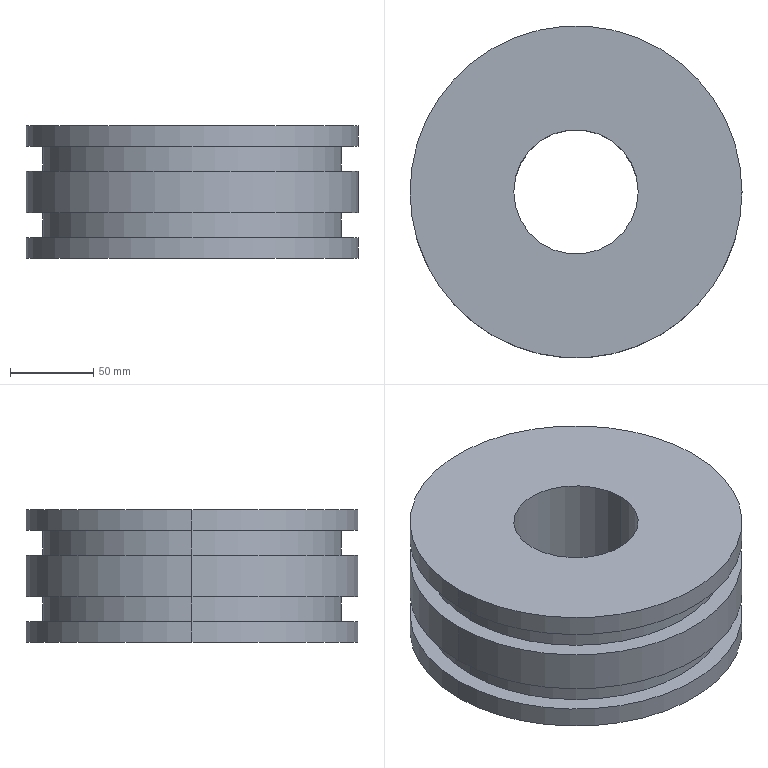Part | SolidWorks | features Extrusion 1, ICE 1, MirrorPattern 1 | 1 solid | 18 faces | box 200 x 200 x 80 mm | volume 1980774 mm3 | cylinder 12 | plane 6 | commonest cylinder face diameters 200 x6 180 x4 75 x2
STEP:
#1=CARTESIAN_POINT('',(90.,0.,-12.5));
#2=VERTEX_POINT('',#1);
#3=CARTESIAN_POINT('',(-90.,0.,-12.5));
#4=VERTEX_POINT('',#3);
#5=CARTESIAN_POINT('',(0.,0.,-12.5));
#6=DIRECTION('',(0.,0.,1.));
#7=DIRECTION('',(1.,0.,0.));
#8=AXIS2_PLACEMENT_3D('',#5,#6,#7);
#9=CIRCLE('',#8,90.);
#10=EDGE_CURVE('',#2,#4,#9,.T.);
#11=ORIENTED_EDGE('',*,*,#10,.F.);
#12=CARTESIAN_POINT('',(90.,0.,-27.5));
#13=VERTEX_POINT('',#12);
#14=CARTESIAN_POINT('',(90.,0.,-12.5));
#15=DIRECTION('',(0.,0.,-1.));
#16=VECTOR('',#15,1000.);
#17=LINE('',#14,#16);
#18=EDGE_CURVE('',#2,#13,#17,.T.);
#19=ORIENTED_EDGE('',*,*,#18,.T.);
#20=CARTESIAN_POINT('',(-90.,0.,-27.5));
#21=VERTEX_POINT('',#20);
#22=CARTESIAN_POINT('',(0.,0.,-27.5));
#23=DIRECTION('',(0.,0.,1.));
#24=DIRECTION('',(1.,0.,0.));
#25=AXIS2_PLACEMENT_3D('',#22,#23,#24);
#26=CIRCLE('',#25,90.);
#27=EDGE_CURVE('',#13,#21,#26,.T.);
#28=ORIENTED_EDGE('',*,*,#27,.T.);
#29=CARTESIAN_POINT('',(-90.,0.,-12.5));
#30=DIRECTION('',(0.,0.,-1.));
#31=VECTOR('',#30,1000.);
#32=LINE('',#29,#31);
#33=EDGE_CURVE('',#4,#21,#32,.T.);
#34=ORIENTED_EDGE('',*,*,#33,.F.);
#35=EDGE_LOOP('',(#11,#19,#28,#34));
#36=FACE_OUTER_BOUND('',#35,.T.);
#37=CARTESIAN_POINT('',(0.,0.,-12.5));
#38=DIRECTION('',(0.,0.,-1.));
#39=DIRECTION('',(-1.,0.,0.));
#40=AXIS2_PLACEMENT_3D('',#37,#38,#39);
#41=CYLINDRICAL_SURFACE('',#40,90.);
#42=ADVANCED_FACE('',(#36),#41,.T.);
#43=CARTESIAN_POINT('',(90.,0.,12.5));
#44=VERTEX_POINT('',#43);
#45=CARTESIAN_POINT('',(-90.,0.,12.5));
#46=VERTEX_POINT('',#45);
#47=CARTESIAN_POINT('',(0.,0.,12.5));
#48=DIRECTION('',(0.,0.,1.));
#49=DIRECTION('',(1.,0.,0.));
#50=AXIS2_PLACEMENT_3D('',#47,#48,#49);
#51=CIRCLE('',#50,90.);
#52=EDGE_CURVE('',#44,#46,#51,.T.);
#53=ORIENTED_EDGE('',*,*,#52,.T.);
#54=CARTESIAN_POINT('',(-90.,0.,27.5));
#55=VERTEX_POINT('',#54);
#56=CARTESIAN_POINT('',(-90.,0.,12.5));
#57=DIRECTION('',(0.,0.,1.));
#58=VECTOR('',#57,1000.);
#59=LINE('',#56,#58);
#60=EDGE_CURVE('',#46,#55,#59,.T.);
#61=ORIENTED_EDGE('',*,*,#60,.T.);
#62=CARTESIAN_POINT('',(90.,0.,27.5));
#63=VERTEX_POINT('',#62);
#64=CARTESIAN_POINT('',(0.,0.,27.5));
#65=DIRECTION('',(0.,0.,1.));
#66=DIRECTION('',(1.,0.,0.));
#67=AXIS2_PLACEMENT_3D('',#64,#65,#66);
#68=CIRCLE('',#67,90.);
#69=EDGE_CURVE('',#63,#55,#68,.T.);
#70=ORIENTED_EDGE('',*,*,#69,.F.);
#71=CARTESIAN_POINT('',(90.,0.,12.5));
#72=DIRECTION('',(0.,0.,1.));
#73=VECTOR('',#72,1000.);
#74=LINE('',#71,#73);
#75=EDGE_CURVE('',#44,#63,#74,.T.);
#76=ORIENTED_EDGE('',*,*,#75,.F.);
#77=EDGE_LOOP('',(#53,#61,#70,#76));
#78=FACE_OUTER_BOUND('',#77,.T.);
#79=CARTESIAN_POINT('',(0.,0.,12.5));
#80=DIRECTION('',(0.,0.,1.));
#81=DIRECTION('',(1.,0.,0.));
#82=AXIS2_PLACEMENT_3D('',#79,#80,#81);
#83=CYLINDRICAL_SURFACE('',#82,90.);
#84=ADVANCED_FACE('',(#78),#83,.T.);
#85=CARTESIAN_POINT('',(-37.5,0.,40.));
#86=VERTEX_POINT('',#85);
#87=CARTESIAN_POINT('',(37.5,0.,40.));
#88=VERTEX_POINT('',#87);
#89=CARTESIAN_POINT('',(0.,0.,40.));
#90=DIRECTION('',(0.,0.,1.));
#91=DIRECTION('',(1.,0.,0.));
#92=AXIS2_PLACEMENT_3D('',#89,#90,#91);
#93=CIRCLE('',#92,37.5);
#94=EDGE_CURVE('',#86,#88,#93,.T.);
#95=ORIENTED_EDGE('',*,*,#94,.T.);
#96=CARTESIAN_POINT('',(37.5,0.,-40.));
#97=VERTEX_POINT('',#96);
#98=CARTESIAN_POINT('',(37.5,0.,40.));
#99=DIRECTION('',(0.,0.,-1.));
#100=VECTOR('',#99,1000.);
#101=LINE('',#98,#100);
#102=EDGE_CURVE('',#88,#97,#101,.T.);
#103=ORIENTED_EDGE('',*,*,#102,.T.);
#104=CARTESIAN_POINT('',(-37.5,0.,-40.));
#105=VERTEX_POINT('',#104);
#106=CARTESIAN_POINT('',(0.,0.,-40.));
#107=DIRECTION('',(0.,0.,1.));
#108=DIRECTION('',(1.,0.,0.));
#109=AXIS2_PLACEMENT_3D('',#106,#107,#108);
#110=CIRCLE('',#109,37.5);
#111=EDGE_CURVE('',#105,#97,#110,.T.);
#112=ORIENTED_EDGE('',*,*,#111,.F.);
#113=CARTESIAN_POINT('',(-37.5,0.,40.));
#114=DIRECTION('',(0.,0.,-1.));
#115=VECTOR('',#114,1000.);
#116=LINE('',#113,#115);
#117=EDGE_CURVE('',#86,#105,#116,.T.);
#118=ORIENTED_EDGE('',*,*,#117,.F.);
#119=EDGE_LOOP('',(#95,#103,#112,#118));
#120=FACE_OUTER_BOUND('',#119,.T.);
#121=CARTESIAN_POINT('',(0.,0.,40.));
#122=DIRECTION('',(0.,0.,-1.));
#123=DIRECTION('',(-1.,0.,0.));
#124=AXIS2_PLACEMENT_3D('',#121,#122,#123);
#125=CYLINDRICAL_SURFACE('',#124,37.5);
#126=ADVANCED_FACE('',(#120),#125,.F.);
#127=CARTESIAN_POINT('',(100.,0.,40.));
#128=VERTEX_POINT('',#127);
#129=CARTESIAN_POINT('',(-100.,0.,40.));
#130=VERTEX_POINT('',#129);
#131=CARTESIAN_POINT('',(0.,0.,40.));
#132=DIRECTION('',(0.,0.,1.));
#133=DIRECTION('',(1.,0.,0.));
#134=AXIS2_PLACEMENT_3D('',#131,#132,#133);
#135=CIRCLE('',#134,100.);
#136=EDGE_CURVE('',#128,#130,#135,.T.);
#137=ORIENTED_EDGE('',*,*,#136,.F.);
#138=CARTESIAN_POINT('',(100.,0.,27.5));
#139=VERTEX_POINT('',#138);
#140=CARTESIAN_POINT('',(100.,0.,40.));
#141=DIRECTION('',(0.,0.,-1.));
#142=VECTOR('',#141,1000.);
#143=LINE('',#140,#142);
#144=EDGE_CURVE('',#128,#139,#143,.T.);
#145=ORIENTED_EDGE('',*,*,#144,.T.);
#146=CARTESIAN_POINT('',(-100.,0.,27.5));
#147=VERTEX_POINT('',#146);
#148=CARTESIAN_POINT('',(0.,0.,27.5));
#149=DIRECTION('',(0.,0.,1.));
#150=DIRECTION('',(1.,0.,0.));
#151=AXIS2_PLACEMENT_3D('',#148,#149,#150);
#152=CIRCLE('',#151,100.);
#153=EDGE_CURVE('',#139,#147,#152,.T.);
#154=ORIENTED_EDGE('',*,*,#153,.T.);
#155=CARTESIAN_POINT('',(-100.,0.,40.));
#156=DIRECTION('',(0.,0.,-1.));
#157=VECTOR('',#156,1000.);
#158=LINE('',#155,#157);
#159=EDGE_CURVE('',#130,#147,#158,.T.);
#160=ORIENTED_EDGE('',*,*,#159,.F.);
#161=EDGE_LOOP('',(#137,#145,#154,#160));
#162=FACE_OUTER_BOUND('',#161,.T.);
#163=CARTESIAN_POINT('',(0.,0.,40.));
#164=DIRECTION('',(0.,0.,-1.));
#165=DIRECTION('',(-1.,0.,0.));
#166=AXIS2_PLACEMENT_3D('',#163,#164,#165);
#167=CYLINDRICAL_SURFACE('',#166,100.);
#168=ADVANCED_FACE('',(#162),#167,.T.);
#169=CARTESIAN_POINT('',(100.,0.,-27.5));
#170=VERTEX_POINT('',#169);
#171=CARTESIAN_POINT('',(-100.,0.,-27.5));
#172=VERTEX_POINT('',#171);
#173=CARTESIAN_POINT('',(0.,0.,-27.5));
#174=DIRECTION('',(0.,0.,1.));
#175=DIRECTION('',(1.,0.,0.));
#176=AXIS2_PLACEMENT_3D('',#173,#174,#175);
#177=CIRCLE('',#176,100.);
#178=EDGE_CURVE('',#170,#172,#177,.T.);
#179=ORIENTED_EDGE('',*,*,#178,.F.);
#180=CARTESIAN_POINT('',(100.,0.,-40.));
#181=VERTEX_POINT('',#180);
#182=CARTESIAN_POINT('',(100.,0.,40.));
#183=DIRECTION('',(0.,0.,-1.));
#184=VECTOR('',#183,1000.);
#185=LINE('',#182,#184);
#186=EDGE_CURVE('',#170,#181,#185,.T.);
#187=ORIENTED_EDGE('',*,*,#186,.T.);
#188=CARTESIAN_POINT('',(-100.,0.,-40.));
#189=VERTEX_POINT('',#188);
#190=CARTESIAN_POINT('',(0.,0.,-40.));
#191=DIRECTION('',(0.,0.,1.));
#192=DIRECTION('',(1.,0.,0.));
#193=AXIS2_PLACEMENT_3D('',#190,#191,#192);
#194=CIRCLE('',#193,100.);
#195=EDGE_CURVE('',#181,#189,#194,.T.);
#196=ORIENTED_EDGE('',*,*,#195,.T.);
#197=CARTESIAN_POINT('',(-100.,0.,40.));
#198=DIRECTION('',(0.,0.,-1.));
#199=VECTOR('',#198,1000.);
#200=LINE('',#197,#199);
#201=EDGE_CURVE('',#172,#189,#200,.T.);
#202=ORIENTED_EDGE('',*,*,#201,.F.);
#203=EDGE_LOOP('',(#179,#187,#196,#202));
#204=FACE_OUTER_BOUND('',#203,.T.);
#205=CARTESIAN_POINT('',(0.,0.,40.));
#206=DIRECTION('',(0.,0.,-1.));
#207=DIRECTION('',(-1.,0.,0.));
#208=AXIS2_PLACEMENT_3D('',#205,#206,#207);
#209=CYLINDRICAL_SURFACE('',#208,100.);
#210=ADVANCED_FACE('',(#204),#209,.T.);
#211=CARTESIAN_POINT('',(100.,0.,12.5));
#212=VERTEX_POINT('',#211);
#213=CARTESIAN_POINT('',(-100.,0.,12.5));
#214=VERTEX_POINT('',#213);
#215=CARTESIAN_POINT('',(0.,0.,12.5));
#216=DIRECTION('',(0.,0.,1.));
#217=DIRECTION('',(1.,0.,0.));
#218=AXIS2_PLACEMENT_3D('',#215,#216,#217);
#219=CIRCLE('',#218,100.);
#220=EDGE_CURVE('',#212,#214,#219,.T.);
#221=ORIENTED_EDGE('',*,*,#220,.F.);
#222=CARTESIAN_POINT('',(100.,0.,-12.5));
#223=VERTEX_POINT('',#222);
#224=CARTESIAN_POINT('',(100.,0.,40.));
#225=DIRECTION('',(0.,0.,-1.));
#226=VECTOR('',#225,1000.);
#227=LINE('',#224,#226);
#228=EDGE_CURVE('',#212,#223,#227,.T.);
#229=ORIENTED_EDGE('',*,*,#228,.T.);
#230=CARTESIAN_POINT('',(-100.,0.,-12.5));
#231=VERTEX_POINT('',#230);
#232=CARTESIAN_POINT('',(0.,0.,-12.5));
#233=DIRECTION('',(0.,0.,1.));
#234=DIRECTION('',(1.,0.,0.));
#235=AXIS2_PLACEMENT_3D('',#232,#233,#234);
#236=CIRCLE('',#235,100.);
#237=EDGE_CURVE('',#223,#231,#236,.T.);
#238=ORIENTED_EDGE('',*,*,#237,.T.);
#239=CARTESIAN_POINT('',(-100.,0.,40.));
#240=DIRECTION('',(0.,0.,-1.));
#241=VECTOR('',#240,1000.);
#242=LINE('',#239,#241);
#243=EDGE_CURVE('',#214,#231,#242,.T.);
#244=ORIENTED_EDGE('',*,*,#243,.F.);
#245=EDGE_LOOP('',(#221,#229,#238,#244));
#246=FACE_OUTER_BOUND('',#245,.T.);
#247=CARTESIAN_POINT('',(0.,0.,40.));
#248=DIRECTION('',(0.,0.,-1.));
#249=DIRECTION('',(-1.,0.,0.));
#250=AXIS2_PLACEMENT_3D('',#247,#248,#249);
#251=CYLINDRICAL_SURFACE('',#250,100.);
#252=ADVANCED_FACE('',(#246),#251,.T.);
#253=ORIENTED_EDGE('',*,*,#228,.F.);
#254=CARTESIAN_POINT('',(0.,0.,12.5));
#255=DIRECTION('',(0.,0.,1.));
#256=DIRECTION('',(1.,0.,0.));
#257=AXIS2_PLACEMENT_3D('',#254,#255,#256);
#258=CIRCLE('',#257,100.);
#259=EDGE_CURVE('',#214,#212,#258,.T.);
#260=ORIENTED_EDGE('',*,*,#259,.F.);
#261=ORIENTED_EDGE('',*,*,#243,.T.);
#262=CARTESIAN_POINT('',(0.,0.,-12.5));
#263=DIRECTION('',(0.,0.,1.));
#264=DIRECTION('',(1.,0.,0.));
#265=AXIS2_PLACEMENT_3D('',#262,#263,#264);
#266=CIRCLE('',#265,100.);
#267=EDGE_CURVE('',#231,#223,#266,.T.);
#268=ORIENTED_EDGE('',*,*,#267,.T.);
#269=EDGE_LOOP('',(#253,#260,#261,#268));
#270=FACE_OUTER_BOUND('',#269,.T.);
#271=CARTESIAN_POINT('',(0.,0.,40.));
#272=DIRECTION('',(0.,0.,-1.));
#273=DIRECTION('',(-1.,0.,0.));
#274=AXIS2_PLACEMENT_3D('',#271,#272,#273);
#275=CYLINDRICAL_SURFACE('',#274,100.);
#276=ADVANCED_FACE('',(#270),#275,.T.);
#277=ORIENTED_EDGE('',*,*,#186,.F.);
#278=CARTESIAN_POINT('',(0.,0.,-27.5));
#279=DIRECTION('',(0.,0.,1.));
#280=DIRECTION('',(1.,0.,0.));
#281=AXIS2_PLACEMENT_3D('',#278,#279,#280);
#282=CIRCLE('',#281,100.);
#283=EDGE_CURVE('',#172,#170,#282,.T.);
#284=ORIENTED_EDGE('',*,*,#283,.F.);
#285=ORIENTED_EDGE('',*,*,#201,.T.);
#286=CARTESIAN_POINT('',(0.,0.,-40.));
#287=DIRECTION('',(0.,0.,1.));
#288=DIRECTION('',(1.,0.,0.));
#289=AXIS2_PLACEMENT_3D('',#286,#287,#288);
#290=CIRCLE('',#289,100.);
#291=EDGE_CURVE('',#189,#181,#290,.T.);
#292=ORIENTED_EDGE('',*,*,#291,.T.);
#293=EDGE_LOOP('',(#277,#284,#285,#292));
#294=FACE_OUTER_BOUND('',#293,.T.);
#295=CARTESIAN_POINT('',(0.,0.,40.));
#296=DIRECTION('',(0.,0.,-1.));
#297=DIRECTION('',(-1.,0.,0.));
#298=AXIS2_PLACEMENT_3D('',#295,#296,#297);
#299=CYLINDRICAL_SURFACE('',#298,100.);
#300=ADVANCED_FACE('',(#294),#299,.T.);
#301=CARTESIAN_POINT('',(0.,0.,40.));
#302=DIRECTION('',(0.,0.,1.));
#303=DIRECTION('',(1.,0.,0.));
#304=AXIS2_PLACEMENT_3D('',#301,#302,#303);
#305=CIRCLE('',#304,100.);
#306=EDGE_CURVE('',#130,#128,#305,.T.);
#307=ORIENTED_EDGE('',*,*,#306,.T.);
#308=ORIENTED_EDGE('',*,*,#136,.T.);
#309=EDGE_LOOP('',(#307,#308));
#310=FACE_OUTER_BOUND('',#309,.T.);
#311=ORIENTED_EDGE('',*,*,#94,.F.);
#312=CARTESIAN_POINT('',(0.,0.,40.));
#313=DIRECTION('',(0.,0.,1.));
#314=DIRECTION('',(1.,0.,0.));
#315=AXIS2_PLACEMENT_3D('',#312,#313,#314);
#316=CIRCLE('',#315,37.5);
#317=EDGE_CURVE('',#88,#86,#316,.T.);
#318=ORIENTED_EDGE('',*,*,#317,.F.);
#319=EDGE_LOOP('',(#311,#318));
#320=FACE_BOUND('',#319,.T.);
#321=CARTESIAN_POINT('',(0.,0.,40.));
#322=DIRECTION('',(0.,0.,1.));
#323=DIRECTION('',(1.,0.,0.));
#324=AXIS2_PLACEMENT_3D('',#321,#322,#323);
#325=PLANE('',#324);
#326=ADVANCED_FACE('',(#310,#320),#325,.T.);
#327=ORIENTED_EDGE('',*,*,#291,.F.);
#328=ORIENTED_EDGE('',*,*,#195,.F.);
#329=EDGE_LOOP('',(#327,#328));
#330=FACE_OUTER_BOUND('',#329,.T.);
#331=ORIENTED_EDGE('',*,*,#111,.T.);
#332=CARTESIAN_POINT('',(0.,0.,-40.));
#333=DIRECTION('',(0.,0.,1.));
#334=DIRECTION('',(1.,0.,0.));
#335=AXIS2_PLACEMENT_3D('',#332,#333,#334);
#336=CIRCLE('',#335,37.5);
#337=EDGE_CURVE('',#97,#105,#336,.T.);
#338=ORIENTED_EDGE('',*,*,#337,.T.);
#339=EDGE_LOOP('',(#331,#338));
#340=FACE_BOUND('',#339,.T.);
#341=CARTESIAN_POINT('',(0.,0.,-40.));
#342=DIRECTION('',(0.,0.,1.));
#343=DIRECTION('',(1.,0.,0.));
#344=AXIS2_PLACEMENT_3D('',#341,#342,#343);
#345=PLANE('',#344);
#346=ADVANCED_FACE('',(#330,#340),#345,.F.);
#347=ORIENTED_EDGE('',*,*,#144,.F.);
#348=ORIENTED_EDGE('',*,*,#306,.F.);
#349=ORIENTED_EDGE('',*,*,#159,.T.);
#350=CARTESIAN_POINT('',(0.,0.,27.5));
#351=DIRECTION('',(0.,0.,1.));
#352=DIRECTION('',(1.,0.,0.));
#353=AXIS2_PLACEMENT_3D('',#350,#351,#352);
#354=CIRCLE('',#353,100.);
#355=EDGE_CURVE('',#147,#139,#354,.T.);
#356=ORIENTED_EDGE('',*,*,#355,.T.);
#357=EDGE_LOOP('',(#347,#348,#349,#356));
#358=FACE_OUTER_BOUND('',#357,.T.);
#359=CARTESIAN_POINT('',(0.,0.,40.));
#360=DIRECTION('',(0.,0.,-1.));
#361=DIRECTION('',(-1.,0.,0.));
#362=AXIS2_PLACEMENT_3D('',#359,#360,#361);
#363=CYLINDRICAL_SURFACE('',#362,100.);
#364=ADVANCED_FACE('',(#358),#363,.T.);
#365=ORIENTED_EDGE('',*,*,#102,.F.);
#366=ORIENTED_EDGE('',*,*,#317,.T.);
#367=ORIENTED_EDGE('',*,*,#117,.T.);
#368=ORIENTED_EDGE('',*,*,#337,.F.);
#369=EDGE_LOOP('',(#365,#366,#367,#368));
#370=FACE_OUTER_BOUND('',#369,.T.);
#371=CARTESIAN_POINT('',(0.,0.,40.));
#372=DIRECTION('',(0.,0.,-1.));
#373=DIRECTION('',(-1.,0.,0.));
#374=AXIS2_PLACEMENT_3D('',#371,#372,#373);
#375=CYLINDRICAL_SURFACE('',#374,37.5);
#376=ADVANCED_FACE('',(#370),#375,.F.);
#377=ORIENTED_EDGE('',*,*,#52,.F.);
#378=CARTESIAN_POINT('',(0.,0.,12.5));
#379=DIRECTION('',(0.,0.,1.));
#380=DIRECTION('',(1.,0.,0.));
#381=AXIS2_PLACEMENT_3D('',#378,#379,#380);
#382=CIRCLE('',#381,90.);
#383=EDGE_CURVE('',#46,#44,#382,.T.);
#384=ORIENTED_EDGE('',*,*,#383,.F.);
#385=EDGE_LOOP('',(#377,#384));
#386=FACE_BOUND('',#385,.T.);
#387=ORIENTED_EDGE('',*,*,#259,.T.);
#388=ORIENTED_EDGE('',*,*,#220,.T.);
#389=EDGE_LOOP('',(#387,#388));
#390=FACE_OUTER_BOUND('',#389,.T.);
#391=CARTESIAN_POINT('',(0.,0.,12.5));
#392=DIRECTION('',(0.,0.,1.));
#393=DIRECTION('',(1.,0.,0.));
#394=AXIS2_PLACEMENT_3D('',#391,#392,#393);
#395=PLANE('',#394);
#396=ADVANCED_FACE('',(#386,#390),#395,.T.);
#397=ORIENTED_EDGE('',*,*,#69,.T.);
#398=CARTESIAN_POINT('',(0.,0.,27.5));
#399=DIRECTION('',(0.,0.,1.));
#400=DIRECTION('',(1.,0.,0.));
#401=AXIS2_PLACEMENT_3D('',#398,#399,#400);
#402=CIRCLE('',#401,90.);
#403=EDGE_CURVE('',#55,#63,#402,.T.);
#404=ORIENTED_EDGE('',*,*,#403,.T.);
#405=EDGE_LOOP('',(#397,#404));
#406=FACE_BOUND('',#405,.T.);
#407=ORIENTED_EDGE('',*,*,#355,.F.);
#408=ORIENTED_EDGE('',*,*,#153,.F.);
#409=EDGE_LOOP('',(#407,#408));
#410=FACE_OUTER_BOUND('',#409,.T.);
#411=CARTESIAN_POINT('',(0.,0.,27.5));
#412=DIRECTION('',(0.,0.,1.));
#413=DIRECTION('',(1.,0.,0.));
#414=AXIS2_PLACEMENT_3D('',#411,#412,#413);
#415=PLANE('',#414);
#416=ADVANCED_FACE('',(#406,#410),#415,.F.);
#417=ORIENTED_EDGE('',*,*,#60,.F.);
#418=ORIENTED_EDGE('',*,*,#383,.T.);
#419=ORIENTED_EDGE('',*,*,#75,.T.);
#420=ORIENTED_EDGE('',*,*,#403,.F.);
#421=EDGE_LOOP('',(#417,#418,#419,#420));
#422=FACE_OUTER_BOUND('',#421,.T.);
#423=CARTESIAN_POINT('',(0.,0.,12.5));
#424=DIRECTION('',(0.,0.,1.));
#425=DIRECTION('',(1.,0.,0.));
#426=AXIS2_PLACEMENT_3D('',#423,#424,#425);
#427=CYLINDRICAL_SURFACE('',#426,90.);
#428=ADVANCED_FACE('',(#422),#427,.T.);
#429=ORIENTED_EDGE('',*,*,#267,.F.);
#430=ORIENTED_EDGE('',*,*,#237,.F.);
#431=EDGE_LOOP('',(#429,#430));
#432=FACE_OUTER_BOUND('',#431,.T.);
#433=CARTESIAN_POINT('',(0.,0.,-12.5));
#434=DIRECTION('',(0.,0.,1.));
#435=DIRECTION('',(1.,0.,0.));
#436=AXIS2_PLACEMENT_3D('',#433,#434,#435);
#437=CIRCLE('',#436,90.);
#438=EDGE_CURVE('',#4,#2,#437,.T.);
#439=ORIENTED_EDGE('',*,*,#438,.T.);
#440=ORIENTED_EDGE('',*,*,#10,.T.);
#441=EDGE_LOOP('',(#439,#440));
#442=FACE_BOUND('',#441,.T.);
#443=CARTESIAN_POINT('',(0.,0.,-12.5));
#444=DIRECTION('',(0.,0.,-1.));
#445=DIRECTION('',(1.,0.,0.));
#446=AXIS2_PLACEMENT_3D('',#443,#444,#445);
#447=PLANE('',#446);
#448=ADVANCED_FACE('',(#432,#442),#447,.T.);
#449=ORIENTED_EDGE('',*,*,#283,.T.);
#450=ORIENTED_EDGE('',*,*,#178,.T.);
#451=EDGE_LOOP('',(#449,#450));
#452=FACE_OUTER_BOUND('',#451,.T.);
#453=CARTESIAN_POINT('',(0.,0.,-27.5));
#454=DIRECTION('',(0.,0.,1.));
#455=DIRECTION('',(1.,0.,0.));
#456=AXIS2_PLACEMENT_3D('',#453,#454,#455);
#457=CIRCLE('',#456,90.);
#458=EDGE_CURVE('',#21,#13,#457,.T.);
#459=ORIENTED_EDGE('',*,*,#458,.F.);
#460=ORIENTED_EDGE('',*,*,#27,.F.);
#461=EDGE_LOOP('',(#459,#460));
#462=FACE_BOUND('',#461,.T.);
#463=CARTESIAN_POINT('',(0.,0.,-27.5));
#464=DIRECTION('',(0.,0.,-1.));
#465=DIRECTION('',(1.,0.,0.));
#466=AXIS2_PLACEMENT_3D('',#463,#464,#465);
#467=PLANE('',#466);
#468=ADVANCED_FACE('',(#452,#462),#467,.F.);
#469=ORIENTED_EDGE('',*,*,#18,.F.);
#470=ORIENTED_EDGE('',*,*,#438,.F.);
#471=ORIENTED_EDGE('',*,*,#33,.T.);
#472=ORIENTED_EDGE('',*,*,#458,.T.);
#473=EDGE_LOOP('',(#469,#470,#471,#472));
#474=FACE_OUTER_BOUND('',#473,.T.);
#475=CARTESIAN_POINT('',(0.,0.,-12.5));
#476=DIRECTION('',(0.,0.,-1.));
#477=DIRECTION('',(-1.,0.,0.));
#478=AXIS2_PLACEMENT_3D('',#475,#476,#477);
#479=CYLINDRICAL_SURFACE('',#478,90.);
#480=ADVANCED_FACE('',(#474),#479,.T.);
#481=CLOSED_SHELL('',(#42,#84,#126,#168,#210,#252,#276,#300,#326,#346,#364,#376,#396,#416,#428,#448,#468,#480));
#482=MANIFOLD_SOLID_BREP('',#481);
#483=CARTESIAN_POINT('',(0.,0.,0.));
#484=DIRECTION('',(0.,0.,1.));
#485=DIRECTION('',(1.,0.,0.));
#486=AXIS2_PLACEMENT_3D('',#483,#484,#485);
#487=(LENGTH_UNIT()NAMED_UNIT(*)SI_UNIT(.MILLI.,.METRE.));
#488=UNCERTAINTY_MEASURE_WITH_UNIT(LENGTH_MEASURE(0.00001),#487,'','');
#489=(NAMED_UNIT(*)PLANE_ANGLE_UNIT()SI_UNIT($,.RADIAN.));
#490=(NAMED_UNIT(*)SI_UNIT($,.STERADIAN.)SOLID_ANGLE_UNIT());
#491=(GEOMETRIC_REPRESENTATION_CONTEXT(3)GLOBAL_UNCERTAINTY_ASSIGNED_CONTEXT((#488))GLOBAL_UNIT_ASSIGNED_CONTEXT((#487,#489,#490))REPRESENTATION_CONTEXT('',''));
#492=ADVANCED_BREP_SHAPE_REPRESENTATION('',(#482,#486),#491);